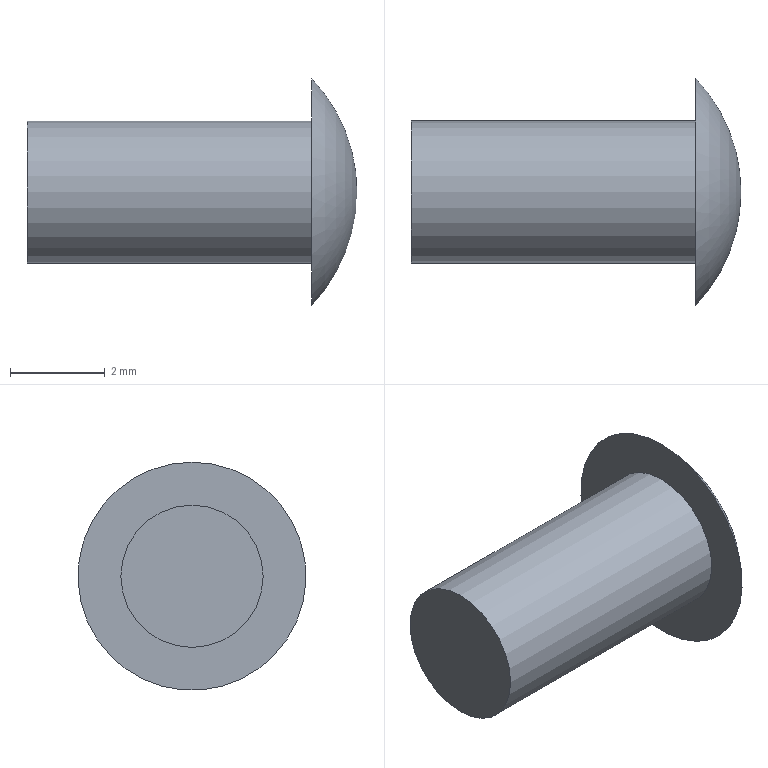Part | STEP file | 1-63 part screw | 1 solid | 4 faces | box 6.956 x 4.807 x 4.807 mm | volume 51.542 mm3 | plane 2 | cylinder 1 | sphere 1 | commonest cylinder face diameters 3 x1
STEP:
#1=CARTESIAN_POINT('',(0.,0.,0.));
#2=DIRECTION('',(0.,0.,1.));
#3=DIRECTION('',(1.,0.,0.));
#4=AXIS2_PLACEMENT_3D('',#1,#2,#3);
#5=CARTESIAN_POINT('',(0.,1.5,0.));
#6=VERTEX_POINT('',#5);
#7=CARTESIAN_POINT('',(0.,0.,0.));
#8=DIRECTION('',(1.,0.,0.));
#9=DIRECTION('',(0.,1.,0.));
#10=AXIS2_PLACEMENT_3D('',#7,#8,#9);
#11=CIRCLE('',#10,1.5);
#12=CARTESIAN_POINT('',(0.,-0.4019,0.));
#13=DIRECTION('',(1.,0.,0.));
#14=DIRECTION('',(0.,1.,0.));
#15=AXIS2_PLACEMENT_3D('',#12,#13,#14);
#16=PLANE('',#15);
#17=CARTESIAN_POINT('',(0.4019,0.));
#18=DIRECTION('',(1.,0.));
#19=AXIS2_PLACEMENT_2D('',#17,#18);
#20=CIRCLE('',#19,1.5);
#21=(GEOMETRIC_REPRESENTATION_CONTEXT(2)PARAMETRIC_REPRESENTATION_CONTEXT()REPRESENTATION_CONTEXT('',''));
#22=DEFINITIONAL_REPRESENTATION('',(#20),#21);
#23=PCURVE('',#16,#22);
#24=CARTESIAN_POINT('',(0.,0.,0.));
#25=DIRECTION('',(1.,0.,0.));
#26=DIRECTION('',(0.,1.,0.));
#27=AXIS2_PLACEMENT_3D('',#24,#25,#26);
#28=CYLINDRICAL_SURFACE('',#27,1.5);
#29=CARTESIAN_POINT('',(0.,0.));
#30=DIRECTION('',(1.,0.));
#31=VECTOR('',#30,1.);
#32=LINE('',#29,#31);
#33=(GEOMETRIC_REPRESENTATION_CONTEXT(2)PARAMETRIC_REPRESENTATION_CONTEXT()REPRESENTATION_CONTEXT('',''));
#34=DEFINITIONAL_REPRESENTATION('',(#32),#33);
#35=PCURVE('',#28,#34);
#36=SURFACE_CURVE('',#11,(#23,#35),.PCURVE_S1.);
#37=EDGE_CURVE('',#6,#6,#36,.T.);
#38=ORIENTED_EDGE('',*,*,#37,.T.);
#39=EDGE_LOOP('',(#38));
#40=FACE_BOUND('',#39,.F.);
#41=ADVANCED_FACE('',(#40),#16,.F.);
#42=ORIENTED_EDGE('',*,*,#37,.T.);
#43=CARTESIAN_POINT('',(6.,1.5,0.));
#44=VERTEX_POINT('',#43);
#45=CARTESIAN_POINT('',(0.,1.5,0.));
#46=DIRECTION('',(1.,0.,0.));
#47=VECTOR('',#46,1.);
#48=LINE('',#45,#47);
#49=CARTESIAN_POINT('',(6.283,0.));
#50=DIRECTION('',(0.,1.));
#51=VECTOR('',#50,1.);
#52=LINE('',#49,#51);
#53=(GEOMETRIC_REPRESENTATION_CONTEXT(2)PARAMETRIC_REPRESENTATION_CONTEXT()REPRESENTATION_CONTEXT('',''));
#54=DEFINITIONAL_REPRESENTATION('',(#52),#53);
#55=PCURVE('',#28,#54);
#56=CARTESIAN_POINT('',(0.,0.));
#57=DIRECTION('',(0.,1.));
#58=VECTOR('',#57,1.);
#59=LINE('',#56,#58);
#60=(GEOMETRIC_REPRESENTATION_CONTEXT(2)PARAMETRIC_REPRESENTATION_CONTEXT()REPRESENTATION_CONTEXT('',''));
#61=DEFINITIONAL_REPRESENTATION('',(#59),#60);
#62=PCURVE('',#28,#61);
#63=SEAM_CURVE('',#48,(#55,#62),.PCURVE_S1.);
#64=EDGE_CURVE('',#6,#44,#63,.T.);
#65=ORIENTED_EDGE('',*,*,#64,.T.);
#66=CARTESIAN_POINT('',(6.,0.,0.));
#67=DIRECTION('',(1.,0.,0.));
#68=DIRECTION('',(0.,1.,0.));
#69=AXIS2_PLACEMENT_3D('',#66,#67,#68);
#70=CIRCLE('',#69,1.5);
#71=CARTESIAN_POINT('',(0.,6.));
#72=DIRECTION('',(1.,0.));
#73=VECTOR('',#72,1.);
#74=LINE('',#71,#73);
#75=(GEOMETRIC_REPRESENTATION_CONTEXT(2)PARAMETRIC_REPRESENTATION_CONTEXT()REPRESENTATION_CONTEXT('',''));
#76=DEFINITIONAL_REPRESENTATION('',(#74),#75);
#77=PCURVE('',#28,#76);
#78=CARTESIAN_POINT('',(6.,0.,0.));
#79=DIRECTION('',(-1.,0.,0.));
#80=DIRECTION('',(0.,0.,1.));
#81=AXIS2_PLACEMENT_3D('',#78,#79,#80);
#82=PLANE('',#81);
#83=CARTESIAN_POINT('',(0.,1.5));
#84=CARTESIAN_POINT('',(2.598,1.5));
#85=CARTESIAN_POINT('',(1.299,-0.75));
#86=CARTESIAN_POINT('',(0.,-3.));
#87=CARTESIAN_POINT('',(-1.299,-0.75));
#88=CARTESIAN_POINT('',(-2.598,1.5));
#89=CARTESIAN_POINT('',(0.,1.5));
#90=(BOUNDED_CURVE()B_SPLINE_CURVE(2,(#83,#84,#85,#86,#87,#88,#89),.UNSPECIFIED.,.T.,.F.)B_SPLINE_CURVE_WITH_KNOTS((1,2,2,2,2,1),(-2.094,0.,2.094,4.189,6.283,8.378),.UNSPECIFIED.)CURVE()GEOMETRIC_REPRESENTATION_ITEM()RATIONAL_B_SPLINE_CURVE((1.,0.5,1.,0.5,1.,0.5,1.))REPRESENTATION_ITEM(''));
#91=(GEOMETRIC_REPRESENTATION_CONTEXT(2)PARAMETRIC_REPRESENTATION_CONTEXT()REPRESENTATION_CONTEXT('',''));
#92=DEFINITIONAL_REPRESENTATION('',(#90),#91);
#93=PCURVE('',#82,#92);
#94=SURFACE_CURVE('',#70,(#77,#93),.PCURVE_S1.);
#95=EDGE_CURVE('',#44,#44,#94,.T.);
#96=ORIENTED_EDGE('',*,*,#95,.F.);
#97=ORIENTED_EDGE('',*,*,#64,.F.);
#98=EDGE_LOOP('',(#42,#65,#96,#97));
#99=FACE_BOUND('',#98,.T.);
#100=ADVANCED_FACE('',(#99),#28,.T.);
#101=CARTESIAN_POINT('',(6.,0.,2.404));
#102=VERTEX_POINT('',#101);
#103=CARTESIAN_POINT('',(6.,0.,0.));
#104=DIRECTION('',(1.,0.,0.));
#105=DIRECTION('',(0.,0.,1.));
#106=AXIS2_PLACEMENT_3D('',#103,#104,#105);
#107=CIRCLE('',#106,2.404);
#108=CARTESIAN_POINT('',(2.404,0.));
#109=CARTESIAN_POINT('',(2.404,-4.163));
#110=CARTESIAN_POINT('',(-1.202,-2.082));
#111=CARTESIAN_POINT('',(-4.807,0.));
#112=CARTESIAN_POINT('',(-1.202,2.082));
#113=CARTESIAN_POINT('',(2.404,4.163));
#114=CARTESIAN_POINT('',(2.404,0.));
#115=(BOUNDED_CURVE()B_SPLINE_CURVE(2,(#108,#109,#110,#111,#112,#113,#114),.UNSPECIFIED.,.T.,.F.)B_SPLINE_CURVE_WITH_KNOTS((1,2,2,2,2,1),(-2.094,0.,2.094,4.189,6.283,8.378),.UNSPECIFIED.)CURVE()GEOMETRIC_REPRESENTATION_ITEM()RATIONAL_B_SPLINE_CURVE((1.,0.5,1.,0.5,1.,0.5,1.))REPRESENTATION_ITEM(''));
#116=(GEOMETRIC_REPRESENTATION_CONTEXT(2)PARAMETRIC_REPRESENTATION_CONTEXT()REPRESENTATION_CONTEXT('',''));
#117=DEFINITIONAL_REPRESENTATION('',(#115),#116);
#118=PCURVE('',#82,#117);
#119=CARTESIAN_POINT('',(3.456,0.,0.));
#120=DIRECTION('',(1.,0.,0.));
#121=DIRECTION('',(0.,0.,1.));
#122=AXIS2_PLACEMENT_3D('',#119,#120,#121);
#123=SPHERICAL_SURFACE('',#122,3.5);
#124=CARTESIAN_POINT('',(0.,0.8138));
#125=CARTESIAN_POINT('',(0.0952,0.8138));
#126=CARTESIAN_POINT('',(0.2856,0.8138));
#127=CARTESIAN_POINT('',(0.5712,0.8138));
#128=CARTESIAN_POINT('',(0.8568,0.8138));
#129=CARTESIAN_POINT('',(1.142,0.8138));
#130=CARTESIAN_POINT('',(1.428,0.8138));
#131=CARTESIAN_POINT('',(1.714,0.8138));
#132=CARTESIAN_POINT('',(1.999,0.8138));
#133=CARTESIAN_POINT('',(2.285,0.8138));
#134=CARTESIAN_POINT('',(2.57,0.8138));
#135=CARTESIAN_POINT('',(2.856,0.8138));
#136=CARTESIAN_POINT('',(3.142,0.8138));
#137=CARTESIAN_POINT('',(3.427,0.8138));
#138=CARTESIAN_POINT('',(3.713,0.8138));
#139=CARTESIAN_POINT('',(3.998,0.8138));
#140=CARTESIAN_POINT('',(4.284,0.8138));
#141=CARTESIAN_POINT('',(4.57,0.8138));
#142=CARTESIAN_POINT('',(4.855,0.8138));
#143=CARTESIAN_POINT('',(5.141,0.8138));
#144=CARTESIAN_POINT('',(5.426,0.8138));
#145=CARTESIAN_POINT('',(5.712,0.8138));
#146=CARTESIAN_POINT('',(5.998,0.8138));
#147=CARTESIAN_POINT('',(6.188,0.8138));
#148=CARTESIAN_POINT('',(6.283,0.8138));
#149=B_SPLINE_CURVE_WITH_KNOTS('',3,(#124,#125,#126,#127,#128,#129,#130,#131,#132,#133,#134,#135,#136,#137,#138,#139,#140,#141,#142,#143,#144,#145,#146,#147,#148),.UNSPECIFIED.,.F.,.F.,(4,1,1,1,1,1,1,1,1,1,1,1,1,1,1,1,1,1,1,1,1,1,4),(0.,0.2856,0.5712,0.8568,1.142,1.428,1.714,1.999,2.285,2.57,2.856,3.142,3.427,3.713,3.998,4.284,4.57,4.855,5.141,5.426,5.712,5.998,6.283),.QUASI_UNIFORM_KNOTS.);
#150=(GEOMETRIC_REPRESENTATION_CONTEXT(2)PARAMETRIC_REPRESENTATION_CONTEXT()REPRESENTATION_CONTEXT('',''));
#151=DEFINITIONAL_REPRESENTATION('',(#149),#150);
#152=PCURVE('',#123,#151);
#153=SURFACE_CURVE('',#107,(#118,#152),.PCURVE_S1.);
#154=EDGE_CURVE('',#102,#102,#153,.T.);
#155=ORIENTED_EDGE('',*,*,#154,.F.);
#156=EDGE_LOOP('',(#155));
#157=FACE_BOUND('',#156,.T.);
#158=ORIENTED_EDGE('',*,*,#95,.T.);
#159=EDGE_LOOP('',(#158));
#160=FACE_BOUND('',#159,.T.);
#161=ADVANCED_FACE('',(#157,#160),#82,.T.);
#162=CARTESIAN_POINT('',(6.956,0.,0.));
#163=VERTEX_POINT('',#162);
#164=CARTESIAN_POINT('',(3.456,0.,0.));
#165=DIRECTION('',(0.,-1.,0.));
#166=DIRECTION('',(1.,0.,0.));
#167=AXIS2_PLACEMENT_3D('',#164,#165,#166);
#168=CIRCLE('',#167,3.5);
#169=CARTESIAN_POINT('',(0.,1.571));
#170=CARTESIAN_POINT('',(0.,1.559));
#171=CARTESIAN_POINT('',(0.,1.536));
#172=CARTESIAN_POINT('',(0.,1.502));
#173=CARTESIAN_POINT('',(0.,1.468));
#174=CARTESIAN_POINT('',(0.,1.433));
#175=CARTESIAN_POINT('',(0.,1.399));
#176=CARTESIAN_POINT('',(0.,1.364));
#177=CARTESIAN_POINT('',(0.,1.33));
#178=CARTESIAN_POINT('',(0.,1.296));
#179=CARTESIAN_POINT('',(0.,1.261));
#180=CARTESIAN_POINT('',(0.,1.227));
#181=CARTESIAN_POINT('',(0.,1.192));
#182=CARTESIAN_POINT('',(0.,1.158));
#183=CARTESIAN_POINT('',(0.,1.123));
#184=CARTESIAN_POINT('',(0.,1.089));
#185=CARTESIAN_POINT('',(0.,1.055));
#186=CARTESIAN_POINT('',(0.,1.02));
#187=CARTESIAN_POINT('',(0.,0.9859));
#188=CARTESIAN_POINT('',(0.,0.9515));
#189=CARTESIAN_POINT('',(0.,0.9171));
#190=CARTESIAN_POINT('',(0.,0.8826));
#191=CARTESIAN_POINT('',(0.,0.8482));
#192=CARTESIAN_POINT('',(0.,0.8253));
#193=CARTESIAN_POINT('',(0.,0.8138));
#194=B_SPLINE_CURVE_WITH_KNOTS('',3,(#169,#170,#171,#172,#173,#174,#175,#176,#177,#178,#179,#180,#181,#182,#183,#184,#185,#186,#187,#188,#189,#190,#191,#192,#193),.UNSPECIFIED.,.F.,.F.,(4,1,1,1,1,1,1,1,1,1,1,1,1,1,1,1,1,1,1,1,1,1,4),(0.,0.03441,0.06882,0.1032,0.1376,0.172,0.2064,0.2409,0.2753,0.3097,0.3441,0.3785,0.4129,0.4473,0.4817,0.5161,0.5505,0.5849,0.6193,0.6537,0.6882,0.7226,0.757),.QUASI_UNIFORM_KNOTS.);
#195=(GEOMETRIC_REPRESENTATION_CONTEXT(2)PARAMETRIC_REPRESENTATION_CONTEXT()REPRESENTATION_CONTEXT('',''));
#196=DEFINITIONAL_REPRESENTATION('',(#194),#195);
#197=PCURVE('',#123,#196);
#198=CARTESIAN_POINT('',(6.283,1.571));
#199=CARTESIAN_POINT('',(6.283,1.559));
#200=CARTESIAN_POINT('',(6.283,1.536));
#201=CARTESIAN_POINT('',(6.283,1.502));
#202=CARTESIAN_POINT('',(6.283,1.468));
#203=CARTESIAN_POINT('',(6.283,1.433));
#204=CARTESIAN_POINT('',(6.283,1.399));
#205=CARTESIAN_POINT('',(6.283,1.364));
#206=CARTESIAN_POINT('',(6.283,1.33));
#207=CARTESIAN_POINT('',(6.283,1.296));
#208=CARTESIAN_POINT('',(6.283,1.261));
#209=CARTESIAN_POINT('',(6.283,1.227));
#210=CARTESIAN_POINT('',(6.283,1.192));
#211=CARTESIAN_POINT('',(6.283,1.158));
#212=CARTESIAN_POINT('',(6.283,1.123));
#213=CARTESIAN_POINT('',(6.283,1.089));
#214=CARTESIAN_POINT('',(6.283,1.055));
#215=CARTESIAN_POINT('',(6.283,1.02));
#216=CARTESIAN_POINT('',(6.283,0.9859));
#217=CARTESIAN_POINT('',(6.283,0.9515));
#218=CARTESIAN_POINT('',(6.283,0.9171));
#219=CARTESIAN_POINT('',(6.283,0.8826));
#220=CARTESIAN_POINT('',(6.283,0.8482));
#221=CARTESIAN_POINT('',(6.283,0.8253));
#222=CARTESIAN_POINT('',(6.283,0.8138));
#223=B_SPLINE_CURVE_WITH_KNOTS('',3,(#198,#199,#200,#201,#202,#203,#204,#205,#206,#207,#208,#209,#210,#211,#212,#213,#214,#215,#216,#217,#218,#219,#220,#221,#222),.UNSPECIFIED.,.F.,.F.,(4,1,1,1,1,1,1,1,1,1,1,1,1,1,1,1,1,1,1,1,1,1,4),(0.,0.03441,0.06882,0.1032,0.1376,0.172,0.2064,0.2409,0.2753,0.3097,0.3441,0.3785,0.4129,0.4473,0.4817,0.5161,0.5505,0.5849,0.6193,0.6537,0.6882,0.7226,0.757),.QUASI_UNIFORM_KNOTS.);
#224=(GEOMETRIC_REPRESENTATION_CONTEXT(2)PARAMETRIC_REPRESENTATION_CONTEXT()REPRESENTATION_CONTEXT('',''));
#225=DEFINITIONAL_REPRESENTATION('',(#223),#224);
#226=PCURVE('',#123,#225);
#227=SEAM_CURVE('',#168,(#197,#226),.PCURVE_S1.);
#228=EDGE_CURVE('',#163,#102,#227,.T.);
#229=ORIENTED_EDGE('',*,*,#228,.T.);
#230=ORIENTED_EDGE('',*,*,#154,.T.);
#231=ORIENTED_EDGE('',*,*,#228,.F.);
#232=EDGE_LOOP('',(#229,#230,#231));
#233=FACE_BOUND('',#232,.T.);
#234=ADVANCED_FACE('',(#233),#123,.T.);
#235=CLOSED_SHELL('',(#41,#100,#161,#234));
#236=MANIFOLD_SOLID_BREP('',#235);
#237=(LENGTH_UNIT()NAMED_UNIT(*)SI_UNIT(.MILLI.,.METRE.));
#238=UNCERTAINTY_MEASURE_WITH_UNIT(LENGTH_MEASURE(0.0000001),#237,'','');
#239=(NAMED_UNIT(*)PLANE_ANGLE_UNIT()SI_UNIT($,.RADIAN.));
#240=(NAMED_UNIT(*)SI_UNIT($,.STERADIAN.)SOLID_ANGLE_UNIT());
#241=(GEOMETRIC_REPRESENTATION_CONTEXT(3)GLOBAL_UNCERTAINTY_ASSIGNED_CONTEXT((#238))GLOBAL_UNIT_ASSIGNED_CONTEXT((#237,#239,#240))REPRESENTATION_CONTEXT('',''));
#242=ADVANCED_BREP_SHAPE_REPRESENTATION('',(#4,#236),#241);